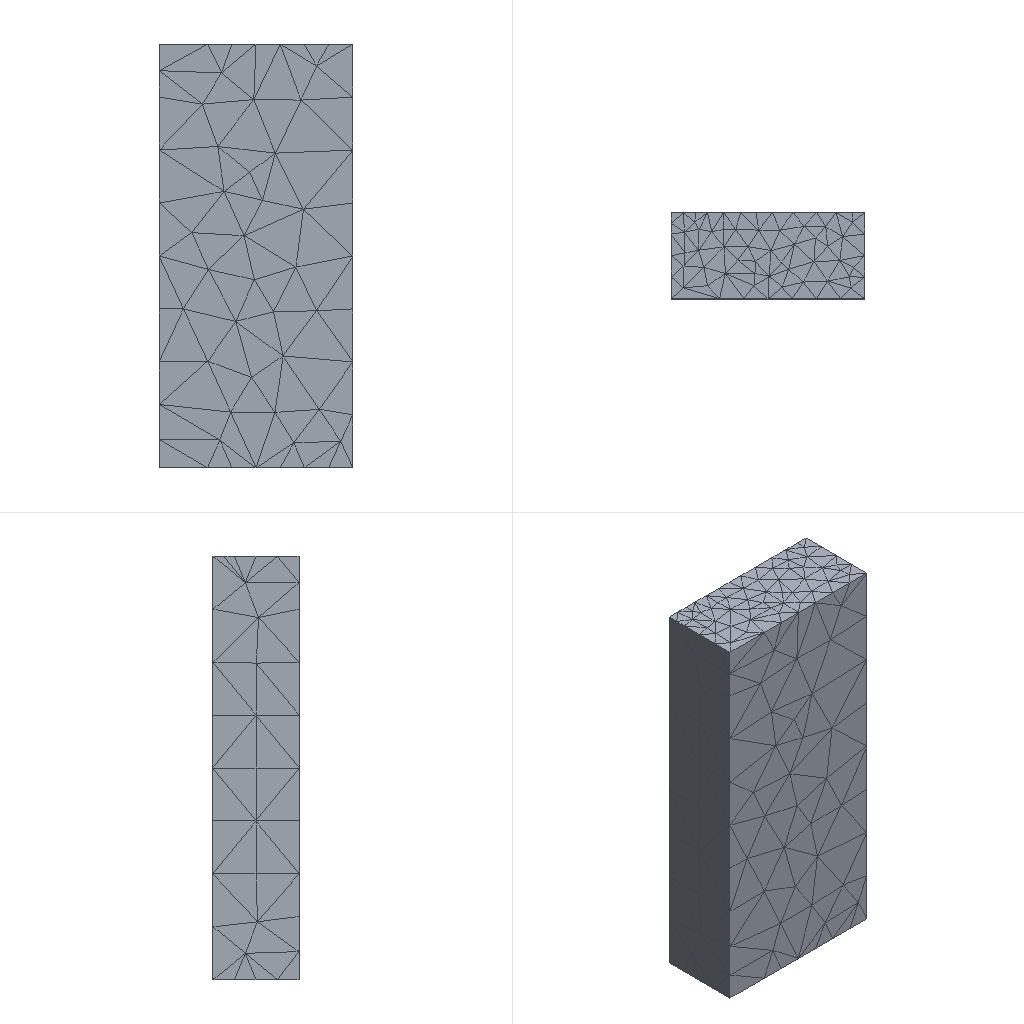Simulation study | ansys electronics desktop
Set-up summary:
category,name,step,type,value,unit,region
solver,ansys_electronics_desktop
units,length mm,,stated,model units
analysis,DESIGN_1,,HFSS Modal Network,design_type=HFSS
setup,Setup1,DESIGN_1,HfssDriven,frequency=10GHz; max_passes=6; max_delta_s=0.02
sweep,Sweep1,Setup1,Discrete,8GHz..12GHz n=9 step=
mesh,nodes,,,n/a (no mesh stored)
mesh,elements,,,n/a (no mesh stored)
material,vacuum,,permittivity,1
load,1,DESIGN_1,wave port,,,faces 8
load,2,DESIGN_1,wave port,,,faces 7
bc,PerfE,DESIGN_1,perfect e,,,"faces 9, 10, 11, 12"
Ansys Electronics Desktop project file, long lists of numbers shortened, first 452 of 1466 lines:
$begin 'AnsoftProject'
	Created='Fri Sep  4 17:09:57 2026'
	Product='ElectronicsDesktop'
	FileOwnedByWorkbench=false
	$begin 'Desktop'
		Version(2026, 1)
		InfrastructureVersion(1, 0)
		$begin 'FactoryHeader'
			$begin 'geometry3deditor'
				KernelVersion(2, 0)
				ProjectContainsGeometry3D='1'
			$end 'geometry3deditor'
		$end 'FactoryHeader'
	$end 'Desktop'
	UsesAdvancedFeatures=false
	PreviewImageDesignId=1
	NextUniqueID=0
	MoveBackwards=false
	$begin 'HFSSEnvironment'
		Version(1, 0)
	$end 'HFSSEnvironment'
	$begin 'PlanarEMEnvironment'
		Version(1, 0)
	$end 'PlanarEMEnvironment'
	$begin 'Q3DEnvironment'
		Version(1, 0)
	$end 'Q3DEnvironment'
	$begin '2DExtractorEnvironment'
		Version(1, 0)
	$end '2DExtractorEnvironment'
	$begin 'NexximEnvironment'
		Version(1, 0)
	$end 'NexximEnvironment'
	$begin 'NexximNetlistEnvironment'
		Version(1, 0)
	$end 'NexximNetlistEnvironment'
	$begin 'EmitEnvironment'
		Version(1, 0)
	$end 'EmitEnvironment'
	$begin 'Maxwell3DEnvironment'
		Version(1, 0)
	$end 'Maxwell3DEnvironment'
	$begin 'Maxwell2DEnvironment'
		Version(1, 0)
	$end 'Maxwell2DEnvironment'
	$begin 'RMxprtEnvironment'
		Version(1, 0)
	$end 'RMxprtEnvironment'
	$begin 'MaxCirEnvironment'
		Version(1, 0)
	$end 'MaxCirEnvironment'
	$begin 'SimplorerEnvironment'
		Version(1, 0)
	$end 'SimplorerEnvironment'
	$begin 'IcepakEnvironment'
		Version(1, 0)
	$end 'IcepakEnvironment'
	$begin 'IcepakFEAEnvironment'
		Version(1, 0)
	$end 'IcepakFEAEnvironment'
	$begin 'SchematicEnvironment'
		Version(1, 0)
	$end 'SchematicEnvironment'
	$begin 'geometry3deditor'
		Version(1, 0)
	$end 'geometry3deditor'
	ReadVersion=12
	$begin 'DesignMgrEnvironment'
		CompInstCounter=1
		GPortCounter=0
		NetCounter=0
		Alias('Ieee;Simplorer Elements\\Ieee', 'Std;Simplorer Elements\\Std', 'Basic_VHDLAMS;Simplorer Elements\\Basic Elements VHDLAMS\\Basic Elements VHDLAMS', 'Digital_Elements;Simplorer Elements\\Digital Elements\\Digital Elements', 'Transformations;Simplorer Elements\\Tools\\Transformations\\Transformations', 'HEV_VHDLAMS;Simplorer Elements\\HEV VHDLAMS\\HEV VHDLAMS', 'automotive_vda;Simplorer Elem
	$end 'DesignMgrEnvironment'
	$begin 'ProjectDatasets'
		NextUniqueID=0
		MoveBackwards=false
		DatasetType='ProjectDatasetType'
		$begin 'DatasetDefinitions'
		$end 'DatasetDefinitions'
	$end 'ProjectDatasets'
	VariableOrders[0:]
	$begin 'Definitions'
		$begin 'Materials'
			$begin 'vacuum'
				CoordinateSystemType='Cartesian'
				BulkOrSurfaceType=1
				$begin 'PhysicsTypes'
					set('Electromagnetic')
				$end 'PhysicsTypes'
				$begin 'AttachedData'
					$begin 'MatAppearanceData'
						property_data='appearance_data'
						Red=230
						Green=230
						Blue=230
						Transparency=0.95
					$end 'MatAppearanceData'
				$end 'AttachedData'
				permittivity='1'
				ModTime=1499970477
				Library='Materials'
				LibLocation='SysLibrary'
				ModSinceLib=false
			$end 'vacuum'
		$end 'Materials'
		$begin 'SurfaceMaterials'
			$begin 'Steel-oxidised-surface'
				CoordinateSystemType='Cartesian'
				BulkOrSurfaceType=2
				$begin 'PhysicsTypes'
					set('Thermal')
				$end 'PhysicsTypes'
				surface_emissivity='0.8'
				ModTime=1461288057
				Library='SurfaceMaterials'
				LibLocation='SysLibrary'
				ModSinceLib=false
			$end 'Steel-oxidised-surface'
		$end 'SurfaceMaterials'
		$begin 'Scripts'
		$end 'Scripts'
		$begin 'AnsysComponents'
			NextUniqueID=0
			MoveBackwards=false
			$begin 'AnsysComponentDefinitions'
			$end 'AnsysComponentDefinitions'
		$end 'AnsysComponents'
		$begin 'Symbols'
			$begin 'DESIGN_1'
				ModTime=1788512998
				Library=''
				ModSinceLib=false
				LibLocation='Project'
				HighestLevel=1
				Normalize=true
				InitialLevels(0, 1)
				$begin 'Graphics'
					Rect(0, 0, 0, 0, 0.00254, 0.00254, 0.00508, 0.00508, 0, 0, 0)
					Rect(0, 1, 0, 0, 0.0004233, 0.00254, 0.0004233, 0.0004233, 0, 0, 0)
				$end 'Graphics'
			$end 'DESIGN_1'
		$end 'Symbols'
		$begin 'DefInfo'
			DESIGN_1(1002, 0, 0, 0, '', 1788512998, '', 'DESIGN_1', '', '', '', '', '', 'Design.bmp', '', 'Project', '', '', 1788512998, '', 0, 0)
		$end 'DefInfo'
		$begin 'Compdefs'
			$begin 'DESIGN_1'
				Library=''
				CircuitEnv=0
				Refbase='U'
				NumParts=1
				ModSinceLib=true
				$begin 'Properties'
					TextProp('Representation', 'SRD', '', 'DESIGN_1')
					TextProp('Owner', 'SRD', '', 'HFSS')
				$end 'Properties'
				CompExtID=6
				$begin 'Parameters'
					ButtonProp('CosimDefinition', 'D', '', 'Edit', 'Edit', 40501, ButtonPropClientData())
					MenuProp('CoSimulator', 'D', '', 'DefaultNetlist', 0)
				$end 'Parameters'
				$begin 'CosimDefinitions'
					$begin 'CosimDefinition'
						CosimulatorType=4
						CosimDefName='DefaultNetlist'
						IsDefinition=true
						Connect=true
						Data()
						GRef()
					$end 'CosimDefinition'
					DefaultCosim='DefaultNetlist'
				$end 'CosimDefinitions'
			$end 'DESIGN_1'
		$end 'Compdefs'
	$end 'Definitions'
	DesignIDServer=2
	MoveBackwards=false
	$begin 'HFSSModel'
		RepRewriteV2=true
		Name='DESIGN_1'
		DesignID=0
		'Use Advanced DC Extrapolation'=false
		'Use Power S'=false
		'Export FRTM After Simulation'=false
		'Export Rays After Simulation'=false
		'Export After Simulation'=false
		'Allow Material Override'=false
		'Calculate Lossy Dielectrics'=false
		'Perform Minimal validation'=false
		$begin 'TemperatureSettings'
			IncludeTemperatureDependence=false
			EnableFeedback=false
			Temperatures(6, '22cel')
		$end 'TemperatureSettings'
		ObjsEnabledForDeformation()
		'Port Validation Settings'='Standard'
		'Save Adaptive support files'=false
		SolutionType='HFSS Modal Network'
		$begin 'DrivenOptions'
			AutoOpen=false
		$end 'DrivenOptions'
		HasTransientSetups=false
		MaterialDensity=1
		MassOfTissue=1
		VoxelSize=1
		TissueObjectList=-1
		AverageSarMethod=0
		UseAutoDCThickness=true
		HaveZwaveSupport=true
		SolveInsideThreshold=100000
		RequireBodyFaceInfo=false
		$begin 'OutputVariable'
			NextUniqueID=0
			MoveBackwards=false
		$end 'OutputVariable'
		$begin 'ModelSetup'
			$begin 'DesignDatasets'
				NextUniqueID=0
				MoveBackwards=false
				DatasetType='DesignDatasetType'
				$begin 'DatasetDefinitions'
				$end 'DatasetDefinitions'
			$end 'DesignDatasets'
			VariableOrders[0:]
			$begin 'Editor3D Doc Preferences'
				BackgroundColorVersion=1
				'Plane Background'=0
				'Need Lights'=true
				'Ambient Light'=8355711
				'Num Lights'=1
				Light0[4: 16777215, 0.75, -0.15, -0.63]
				Ver=2
			$end 'Editor3D Doc Preferences'
			SnapMode=31
			WorkingCS=1
			$begin 'GeometryCore'
				BlockVersionID=3
				DataVersion=3
				NativeKernel='PARASOLID'
				NativeKernelVersionID=26
				Units='mm'
				ModelExtents=10000
				InstanceID=-1
				$begin 'ValidationOptions'
					EntityCheckLevel='Strict'
					IgnoreUnclassifiedObjects=false
					SkipIntersectionChecks=false
				$end 'ValidationOptions'
				ContainsGeomLinkUDM=false
				$begin 'GeometryOperations'
					BlockVersionID=2
					$begin 'AnsoftRangedIDServerManager'
						$begin 'AnsoftRangedIDServer'
							IDServerObjectTypeID=0
							IDServerRangeMin=0
							IDServerRangeMax=2146483647
							NextUniqueID=36
							MoveBackwards=false
						$end 'AnsoftRangedIDServer'
						$begin 'AnsoftRangedIDServer'
							IDServerObjectTypeID=1
							IDServerRangeMin=2146483648
							IDServerRangeMax=2146485547
							NextUniqueID=2146483654
							MoveBackwards=false
						$end 'AnsoftRangedIDServer'
					$end 'AnsoftRangedIDServerManager'
					StartBackGroundFaceID=2146483648
					$begin 'CoordinateSystems'
					$end 'CoordinateSystems'
					$begin 'OperandCSs'
					$end 'OperandCSs'
					$begin 'SubModelDefinitions'
					$end 'SubModelDefinitions'
					$begin 'Groups'
					$end 'Groups'
					$begin 'UserDefinedModels'
					$end 'UserDefinedModels'
					$begin 'OperandUserDefinedModels'
					$end 'OperandUserDefinedModels'
					$begin 'ToplevelParts'
						$begin 'GeometryPart'
							$begin 'Attributes'
								Name='WG'
								Flags=''
								Color='(230 230 230)'
								Transparency=0.8
								PartCoordinateSystem=1
								UDMId=-1
								GroupId=-1
								MaterialValue='"vacuum"'
								SurfaceMaterialValue='""'
								SolveInside=true
								ShellElement=false
								ShellElementThickness='0mm'
								ReferenceTemperature='20cel'
								IsMaterialEditable=true
								IsSurfaceMaterialEditable=true
								UseMaterialAppearance=false
								IsLightweight=false
								IsAlwaysHidden=false
							$end 'Attributes'
							$begin 'PhysicsAttributes'
								SuppressedForPhysics='False'
								SuppressedForPhysicsEditable=true
							$end 'PhysicsAttributes'
							$begin 'Operations'
								$begin 'Operation'
									OperationType='Box'
									ID=5
									ReferenceCoordSystemID=1
									$begin 'BoxParameters'
										KernelVersion=24
										XPosition='0mm'
										YPosition='0mm'
										ZPosition='0mm'
										XSize='22.86mm'
										YSize='10.16mm'
										ZSize='50mm'
									$end 'BoxParameters'
									ParentPartID=6
									ReferenceUDMID=-1
									IsSuppressed=false
									$begin 'OperationIdentity'
										$begin 'Topology'
											NumLumps=1
											NumShells=1
											NumFaces=6
											NumWires=0
											NumLoops=6
											NumCoedges=24
											NumEdges=12
											NumVertices=8
										$end 'Topology'
										BodyID=6
										StartFaceID=7
										StartEdgeID=13
										StartVertexID=25
										NumNewFaces=6
										NumNewEdges=12
										NumNewVertices=8
										FaceNameAndIDMap()
										EdgeNameAndIDMap()
										VertexNameAndIDMap()
									$end 'OperationIdentity'
								$end 'Operation'
							$end 'Operations'
							$begin 'SubregionDependencyInformation'
								ChildSubregions[0:]
							$end 'SubregionDependencyInformation'
						$end 'GeometryPart'
					$end 'ToplevelParts'
					$begin 'OperandParts'
					$end 'OperandParts'
					$begin 'Planes'
					$end 'Planes'
					$begin 'Points'
					$end 'Points'
					$begin 'GeometryEntityLists'
					$end 'GeometryEntityLists'
					$begin 'CachedNames'
						$begin 'allobjects'
							allobjects(-1)
						$end 'allobjects'
						$begin 'global'
							global(-1)
						$end 'global'
						$begin 'model'
							model(-1)
						$end 'model'
						$begin 'wg'
							wg(-1)
						$end 'wg'
					$end 'CachedNames'
				$end 'GeometryOperations'
				$begin 'GeometryDependencies'
					$begin 'DependencyInformation'
						NumParents=1
						DependencyObject('GeometryBodyOperation', 5)
						DependencyObject('CoordinateSystem', 1)
					$end 'DependencyInformation'
				$end 'GeometryDependencies'
			$end 'GeometryCore'
			$begin 'AssignedEntities'
				AssignedObject[1: 6]
				$begin 'AssignedFace'
					kID=7
					$begin 'FaceData'
						ParentObjectID=6
						NormalValid=false
						$begin 'FaceGeomTopol'
							FaceTopol(1, 4, 4, 4)
							$begin 'FaceGeometry'
								Area=232.258
								FcUVMid(11.43, 5.08, 50)
								$begin 'FcTolVts'
									TolVt(22.86, 0, 50, 5e-07)
									TolVt(22.86, 10.16, 50, 5e-07)
									TolVt(0, 10.16, 50, 5e-07)
									TolVt(0, 0, 50, 5e-07)
								$end 'FcTolVts'
							$end 'FaceGeometry'
						$end 'FaceGeomTopol'
					$end 'FaceData'
				$end 'AssignedFace'
				$begin 'AssignedFace'
					kID=8
					$begin 'FaceData'
						ParentObjectID=6
						NormalValid=false
						$begin 'FaceGeomTopol'
							FaceTopol(1, 4, 4, 4)
							$begin 'FaceGeometry'
								Area=232.258
								FcUVMid(11.43, 5.08, 0)
								$begin 'FcTolVts'
									TolVt(22.86, 0, 0, 5e-07)
									TolVt(0, 0, 0, 5e-07)
									TolVt(0, 10.16, 0, 5e-07)
									TolVt(22.86, 10.16, 0, 5e-07)
								$end 'FcTolVts'
							$end 'FaceGeometry'
						$end 'FaceGeomTopol'
					$end 'FaceData'
				$end 'AssignedFace'
				$begin 'AssignedFace'
					kID=9
					$begin 'FaceData'
						ParentObjectID=6
						NormalValid=false
						$begin 'FaceGeomTopol'
							FaceTopol(1, 4, 4, 4)
							$begin 'FaceGeometry'
								Area=1143
								FcUVMid(11.43, 0, 25)
								$begin 'FcTolVts'
									TolVt(22.86, 0, 50, 5e-07)
									TolVt(0, 0, 50, 5e-07)
									TolVt(0, 0, 0, 5e-07)
									TolVt(22.86, 0, 0, 5e-07)
								$end 'FcTolVts'
							$end 'FaceGeometry'
						$end 'FaceGeomTopol'
					$end 'FaceData'
				$end 'AssignedFace'
				$begin 'AssignedFace'
					kID=10
					$begin 'FaceData'
						ParentObjectID=6
						NormalValid=false
						$begin 'FaceGeomTopol'
							FaceTopol(1, 4, 4, 4)
Last 416 lines:
				$end 'RegularArray'
				$begin 'CustomArray'
					NumCells=0
					$begin 'Cell'
					$end 'Cell'
				$end 'CustomArray'
				$begin 'ParametricArray'
					DesignFrequency='1GHz'
					LayoutType=1
					CenterCellX='0mm'
					CenterCellY='0mm'
					CenterCellZ='0mm'
					SpecifyDesignInWavelength=true
					WidthSpacing='14.99mm'
					WidthSpacingInWavelength='0.05'
					Width='119.917mm'
					WidthInWavelength='0.4'
					LengthSpacing='14.99mm'
					LengthSpacingInWavelength='0.05'
					Length='89.938mm'
					LengthInWavelength='0.3'
					SymmetryType=0
					StaggerAngle='0deg'
					StaggerType=0
					UDirnX='1'
					UDirnY='0'
					UDirnZ='0'
					VDirnX='0'
					VDirnY='1'
					VDirnZ='0'
					WeightType=3
					EdgeTaperX_db='-200'
					CosineExp='1'
					DifferentialType=0
					Behavior='UseScanAngle'
					ScanAnglePhi='45deg'
					ScanAngleTheta='45deg'
					UDirnPhaseShift='0deg'
					VDirnPhaseShift='0deg'
				$end 'ParametricArray'
			$end 'ArraySetup'
			$begin 'NearFieldSetups'
				NextUniqueID=0
				MoveBackwards=false
			$end 'NearFieldSetups'
			RadFieldComputationVersion=1.8
			RadfieldHeaderFile='RAD6E3F2452017885130237.tmp'
			RadPowerMethod=0
		$end 'RadField'
		$begin 'SolutionManager'
			$begin 'SimSetup'
				TypeName='BaseSetup'
				ID=6
				Name='Setup1'
				$begin 'Solution'
					ID=7
					Name='AdaptivePass'
					$begin 'SimDataExtractor'
						IsPortOnly=false
					$end 'SimDataExtractor'
				$end 'Solution'
				$begin 'Solution'
					ID=8
					Name='LastAdaptive'
					$begin 'SimDataExtractor'
						$begin 'Sweeps'
							$begin 'Sweep'
								Variable='Freq'
								Column='10GHz'
								Units='GHz'
							$end 'Sweep'
							$begin 'PostprocessSweep'
								Variable='NormalizedDistance'
								RegularSweep=1
								Units=''
								Minimum=0
								Maximum=1
								Increment=0.01
								CreateIndexedSubsweepFlag=false
							$end 'PostprocessSweep'
							$begin 'PostprocessSweep'
								Variable='Phi'
								RegularSweep=1
								Units='deg'
								Minimum=0
								Maximum=6.283
								Increment=0.08727
								CreateIndexedSubsweepFlag=false
							$end 'PostprocessSweep'
							$begin 'PostprocessSweep'
								Variable='Theta'
								RegularSweep=1
								Units='deg'
								Minimum=0
								Maximum=6.283
								Increment=0.08727
								CreateIndexedSubsweepFlag=false
							$end 'PostprocessSweep'
							$begin 'PostprocessSweep'
								Variable='Phase'
								RegularSweep=1
								Units='deg'
								Minimum=0
								Maximum=6.283
								Increment=0.08727
								CreateIndexedSubsweepFlag=false
							$end 'PostprocessSweep'
						$end 'Sweeps'
						IsPortOnly=false
					$end 'SimDataExtractor'
				$end 'Solution'
				$begin 'Solution'
					ID=14
					Name='Sweep1'
					$begin 'SimDataExtractor'
						IsPortOnly=false
					$end 'SimDataExtractor'
				$end 'Solution'
			$end 'SimSetup'
			$begin 'Version ID Map'
				V=1
				$begin 'Setup'
					N='Setup1'
					V=0
					Soln(N='AdaptivePass', V=0)
					Soln(N='LastAdaptive', V=12)
					Soln(N='Sweep1', V=0)
				$end 'Setup'
				IQM=0
			$end 'Version ID Map'
			$begin 'ID Map'
				$begin 'Setup'
					N='Setup1'
					I=6
					Soln(N='AdaptivePass', I=7)
					Soln(N='LastAdaptive', I=8)
					Soln(N='Sweep1', I=14)
				$end 'Setup'
			$end 'ID Map'
			ValidationCacheHeader=''
		$end 'SolutionManager'
		$begin 'UserDefinedSolutionMgr'
			NextUniqueID=1000000
			MoveBackwards=false
		$end 'UserDefinedSolutionMgr'
		$begin 'DatasetSolutionMgr'
			NextUniqueID=2000000
			MoveBackwards=false
		$end 'DatasetSolutionMgr'
		Notes=$begin_cdata$ $end_cdata$
		$begin 'AnimationSetups'
		$end 'AnimationSetups'
		CacheHeaderFile='HDR6E3F2452017885130238.tmp'
	$end 'HFSSModel'
	$begin 'DataInstances'
		DesignEditor='TopLevel'
		Refdes('0', 'U1')
		$begin 'CompInstances'
			$begin 'Compinst'
				ID='0'
				Status='Status'
				CompName='DESIGN_1'
				GatesInUse()
				$begin 'Properties'
					TextProp('ID', 'SRID', '', '0')
				$end 'Properties'
				$begin 'Parameters'
					MenuProp('CoSimulator', 'OHD', '', 'DefaultNetlist', 0)
					ButtonProp('CosimDefinition', 'OHD', '', 'Edit', 'Edit', 40501, ButtonPropClientData())
				$end 'Parameters'
			$end 'Compinst'
		$end 'CompInstances'
		$begin 'Instance'
			DesignEditor='DESIGN_1'
			ID='0'
			$begin 'HfssDesignInstance'
				DesignInstanceID=1
				$begin 'WindowPosition'
					$begin 'EditorWindow'
						Circuit(Editor3d(View('View Orientation Gadget'=1, WindowPos(3, -1, -1, -8, -31, 26, 26, 1631, 489), OrientationMatrix(0.02344, -0.01353, 0.01914, 0, 0.02344, 0.01353, -0.01914, 0, 0, 0.02706, 0.01914, 0, -0.387, -0.5907, -6.194, 1, 0, -2.542, 2.542, -1, 
					$end 'EditorWindow'
				$end 'WindowPosition'
				$begin 'ReportSetup'
					$begin 'ReportManager'
						$begin 'Reports'
						$end 'Reports'
						NextUniqueID=0
						MoveBackwards=false
						$begin 'NextVersID'
							NextUniqueID=0
							MoveBackwards=false
						$end 'NextVersID'
					$end 'ReportManager'
					$begin 'Reports'
					$end 'Reports'
					$begin 'ReportsWindowInfoList'
					$end 'ReportsWindowInfoList'
				$end 'ReportSetup'
				$begin 'Properties'
				$end 'Properties'
				$begin 'UserDefinedDocument'
					$begin 'Data'
					$end 'Data'
				$end 'UserDefinedDocument'
			$end 'HfssDesignInstance'
		$end 'Instance'
		$begin 'SODInfo'
			$begin 'DESIGN_1'
				$begin 'CosimDefinition'
					CosimDefName='DefaultNetlist'
					$begin 'SODInstanceMap'
					$end 'SODInstanceMap'
					SODComponentList()
				$end 'CosimDefinition'
			$end 'DESIGN_1'
		$end 'SODInfo'
	$end 'DataInstances'
	$begin 'WBSystemIDToDesignInstanceIDMap'
	$end 'WBSystemIDToDesignInstanceIDMap'
	$begin 'WBSysIDSysDetails'
	$end 'WBSysIDSysDetails'
	$begin 'WBConnIDConnDetails'
	$end 'WBConnIDConnDetails'
	$begin 'WBMaterialGuidDetails'
		WBMaterialGuidMap()
	$end 'WBMaterialGuidDetails'
	$begin 'MinervaProjectSettingsBlk'
		MinervaRemoteFilePath=''
		FolderContainerString=''
	$end 'MinervaProjectSettingsBlk'
$end 'AnsoftProject'
$begin 'AllReferencedFilesForProject'
$end 'AllReferencedFilesForProject'
$begin 'ProjectPreview'
	ProductName='ElectronicsDesktop'
	MajorVersion=2026
	MinorVersion=1
	IsEncrypted=false
	Thumbnail64='/9j/4AAQSkZJRgABAQAAAQABAAD/2wBDAAEBAQEBAQEBAQEBAQEBAQEBAQEBAQEBAQEBAQEBAQEBAQE\
BAQICAQECAQEBAgICAgICAgICAQICAgICAgICAgL/2wBDAQEBAQEBAQEBAQECAQEBAgICAgICAgICAg\
ICAgICAgICAgICAgICAgICAgICAgICAgICAgICAgICAgICAgICAgL/wAARCABgAGADASIAAhEBAxEB/\
8QAHwAAAQUBAQEBAQEAAAAAAAAAAAECAwQFBgcICQoL/8QAtRAAAgEDAwIEAwUFBAQAAAF9AQIDAAQR\
BRIhMUEGE1FhByJxFDKBkaEII0KxwRVS0fAkM2JyggkKFhcYGRolJicoKSo0NTY3ODk6Q0RFRkdISUp\
TVFVWV1hZWmNkZWZnaGlqc3R1dnd4eXqDhIWGh4iJipKTlJWWl5iZmqKjpKWmp6ipqrKztLW2t7i5us\
LDxMXGx8jJytLT1NXW19jZ2uHi4+Tl5ufo6erx8vP09fb3+Pn6/8QAHwEAAwEBAQEBAQEBAQAAAAAAA\
AECAwQFBgcICQoL/8QAtREAAgECBAQDBAcFBAQAAQJ3AAECAxEEBSExBhJBUQdhcRMiMoEIFEKRobHB\
CSMzUvAVYnLRChYkNOEl8RcYGRomJygpKjU2Nzg5OkNERUZHSElKU1RVVldYWVpjZGVmZ2hpanN0dXZ\
3eHl6goOEhYaHiImKkpOUlZaXmJmaoqOkpaanqKmqsrO0tba3uLm6wsPExcbHyMnK0tPU1dbX2Nna4u\
Pk5ebn6Onq8vP09fb3+Pn6/9oADAMBAAIRAxEAPwD+rnTfH/7fXxx/aA/bO8I/BT43fsgfB/4Zfsz/A\
LQHgn4F+GdH+KX7HPxo+OvjvxF/bf7IH7LP7SGs+Kdd8b+E/wBvL4e6fHu8QftB6rp1rY2/hyP7PZ+H\
Ld5by6nmkZfQP+Fc/wDBU3/o8j9gD/xWn+0V/wDTYq/Er/goPrX7Z3hTV/2tvHv7EOj/ALQnif4g/C7\
/AILq/Ar4wfEHwV+zvbfETUNY+I3wl+D/APwQr/Zp+J+q/C34h6P8Oo3l8RfDLxT448J+APDtxpWpRz\
aZqur+JtG05oZr+6sIn8I+Cn7Qv/BZf9k74Jfs6eDPFp/aP8YRfDf9nj/gpV4n+OPxJ/ap+HWu6n4Iu\
/G3w21f/gqj4z+BHjX42/tL/Fbw1d3nh3RftvwR/ZEi02bV/FvgvQ7Hwn8RdINpB41sPFtnc+AwD+iz\
/hXP/BU3/o8j9gD/AMVp/tFf/TYqP+Fc/wDBU3/o8j9gD/xWn+0V/wDTYq8t/wCCVXx5+K3x18K/tbD\
4n/FL4s/F2y+FP7Vmi/DX4ZeKvjn8EvCX7PnxWT4f3v7GX7H/AMWbjT/GPwz8I/D7wwmk6gfiP8U/iH\
dq15pMN6YdViiZYbWG1tLb5v8A+Ca+k/GWy/bC/a98RfG34n/tOX2oz/Fz9vKPQ/hr8afgj/wVO8PfD\
nwx8L4f24/E5+COu+Bfj18ev2htR/Zp8Y+HG+CNn4Hk8Mad8Nvh1oHiCHwxrkMdtq81npPi6XWgD7i/\
4Vz/AMFTf+jyP2AP/Faf7RX/ANNio/4Vz/wVN/6PI/YA/wDFaf7RX/02Kv8APS+EuqftaXnhTwt+33q\
kX7SnxA+InwL8SfA+81r9oLxdffEz4weD4/FXww0jwPpPjeX4n/HXx/rmp3eneL7vxz4t+EzaR4eubx\
re60vxZrVtplva6RoKWcf7pfCj/gpF/wAFK/2M/gZ8F/2kvj14++NP7Q37PFpqPg3wl4b8D/GT4ceC/\
h1/wuzwh49+I/8AwVN+Gvgm40/9o+4+Ds/iLxH4h0n4Tfsm/sY/EFdYu7rXtV1/TvjlPqWv3Wo23i/Q\
NXtAD93P2sfFv/BU39l/9lj9pb9pf/hqD9gDxx/wzv8As/8Axk+On/CFf8O7v2ivDP8AwmH/AAqT4de\
I/H//AAi3/CR/8PS9Q/4R/wDtD/hH/sn277BffZPtfn/Y7ny/Jf8AX6v4pfjT/wAFLfi34D/4JRftIf\
Bbxf8AsxftDeNPgD+03pv/AAVT/Zp/Zz/au+L37Qmp/Ev4kSXPjT4tftXeDPhV8L/iloXxRvta8XWet\
eCdGudJ8H3z+J/FE+py2/wtvrjTm1O3tY9/7y/tDf8ABUfxJ4J/a51b9h39lr9lPxN+1n+0N4P8G2Xj\
n4gaEfiz4J+BXhvwzpGo6RoPiG2trHxT48065i8R6ougeKPDl3PHDHHEia1FFFNPPFexWgB+utFfij8\
VP+CtfxU+Ev7Hnjb9p/xj/wAE+/jp4F8U/Cb4r+Fvh58VvhL8XNU1j4Z2GneHPFc2paRZfEr4cfFO5+\
GN9YfFbwyviyPQtLb7FZWyiXXUuHnjtmsZNR9x/bR/4KWaD+zH8Pv2UPE/wt+GX/DQ/i/9svx14N8Lf\
BXwLB46X4eHXdD8ZaNpupWnixddTwhrxkgjvfE/ga1Nulkd58VpKbhBDslAP09or8V/F/8AwVo+JHir\
9oj4+fs9/sY/sQeMP2uNS/Zg1KbQ/jT4iT43fD/4NRaRrdjf6ppGrWHhLQfFWkX1541+za3omsWGLdY\
ria70yRIbZ4ZLWe4/SD9lr496j+0l8HtD+J2t/Bf4xfs/eILy7vtK8QfCz44+CNe8DeNfD2r6a0QuDF\
aa9ptq2u+Hpo54JbLU7eIQXMchR0gu4Lq1twD8Z/Efx6+K/wCzv+1f+3fqWmftd/st/s2+Avj1/wAFV\
v2cP2Xvh1ovxx/Yi/aD/ad8R+Nf2lvib/wS8/YFvvCmjWvjf4Nftf8AgSy8EeGtR0HQBGja1oaadps+\
gXd3qPidYtQtLOz3PBP7ePij43fB34ffEu2/4LA/8EeLf4V/tAeH/iHP8P7X41fsB/HD4M6h8SvCngX\
xT4v+G3xHuLT4afHb/grBoOtaj4cs/EfgvxjYXslxpItZItInlBls2SZ/jT9ur4V/DX9qT4o/t8/ADx\
L8Qf2pPhB4z+GP/BVP4U/tQ+EPiL8Dv+CcH7Z/7bvhy112z/4Iq/sr/BfwXBda/wDs6/Dm80PQPEul+\
L/iHa+I30+61xNVEHhC0im061tdesdWi8Mvv2QPBFj8BvgF+zh4F/a5/wCCiHhr4S/s+ePG+KnhjwBq\
v/BCP/grfrXw81X4i2P7ePj79tDRNc8TfDzRPBujaV4303+xPGWjeDNQ07xPb+IbZh4C03xHoP8Awjd\
3NqWn3wB92fET9mT4Vf8ACl1bxj8T/wDg33+IXwY/Z9ifxJongrw5/wAEU9Y+NWm/Di4+OHxQ1L4QrP\
8AD74UeBP+ClOtXlr4h8a/Gv4Uav4WgttC0l9Q8U+K/hrc6FBDqGsaNLaW3hf7Z3/BUn43WH7Jvxr1L\
wZ+3Z+yr8XH1jRtQ+D2o6H8O/8Aglb+278DNZ0vxl4xk/4RPxh8Mpvjl8UP23db8NfBv9o/w94Y1LWd\
bvPBuv6Xd+MdKt9D+1X3hWK3P2hPqj4RfGFP2d/2HtC/Y2+BHxj/AGxfBOofDD4MeB/hD8CvjZqv/BA\
L/gqV4j8TeCW8K+MvFX9peLfG/hCD4SWGkfEfVrv4QXHgHRoVgj0F4PE3h7W/GF9catD4gtfDOgfnx4\
9/Y8/Zr+Mf/CFzfFTXP2kLe4+H/jbwh8cdM0z4S/8ABBz/AILueE/AvxA/aR+Hsd1o3hj4pfHj4a/FX\
x9480T4rwaj4Mey0zxrOLPSvHvjRbBX1T4jR2whsYADz/8AZs/4JJePfiT8HvhX+zlaf8FTvi58GfGX\
7Rn7OviP9qDU/wBhXVfg38avDGiWfg/Q/EngHwb431Hx54P1v4vaLarpsPxC8Y+C9MTUdU8PWza+0T6\
joNtq+nadPdQ/nD8cP2gvjF4p/wCCXXw//Zh+K3xZ+Eduf2Y/2wp/hzpP7Pk3wu8Taf8AtE2MHh3wN8\
U7yXx9rHxeuPjpdaT4g+Hmk6n401rwy2jW/wAPdPurSZdIaTxE6Qm31D+lj4MeK/gv8BR8DNc+Hus/t\
mWnjP4Cfs3/ALdXwX8HW13/AMEMf+Cry/CTTfFf7Zvx6+Av7QOhaj4d+GWj/Bmzu/CfwG+H2ufBCDw/\
4e+Htp4iNwfCOo6fo1v4w0uTRlvr784vj5+xz8Etc1/9rD4p/Bv4jft3+N/iD+0D8cP2jfjP4B8BftQ\
/8EXf+Cl+s+AfgPqv7WOg/s9WfxX8S/CL4jfDr9iK08UeCPjxoviv9nzwXqfw/wDG11H4hsvB+neDtA\
0ay8HvrUWu+NdfAPFP+CnXj628Q/8ABPX4c/Dz4WfGb9jjxB+z98Mv2h/hbrvhT4N/sw/8Eyv2hv8Ag\
n3Y6LZ/GfwF+074o8D/ABg8AyfF79pjxNovj74G+Kbrw78W7ix1fwt4afRvE+qi61Sx8UytYX9vf+4/\
8FjLT9j1v+ChXxFvPjZN8f8A4FfEjSfCPw/8ReHfjv8ACHS7TUdO8RTaZ8P/AA1/Y9lLZwapPcXHiWN\
0nsbWcR6AYW0uFbvUvsYgnHxz4v8A2y/hp+yd+wT/AMFSvhf4J8La38R9N+L/AMJfAH7GL/Fbw1+zD8\
dv2Z/AXxN1iT4C/HW1/aF+Ofxotfib4OebTP2+biTxtq1j4rn8XXum6/42bwd4f1m08P3Gk+HNZkr6I\
/aG/aN+NPxO+Nf7QXj3XF+Cvgfxv8I/jt49+FHxg8UjT/Fg8FSaj8ANM0fwHD4s8KeFbjWZLryNQi8O\
adM9vqGuSNZRny0mv8JGPpeF8HSx+MxeFqyhGNTDz1lS9rqqlJ3jHnpcskk3z+0goxUnKXLdP8D+kJ4\
gY7wz4c4Q4qweCrZhTo8QYShiKVLGrAxlQxGCzGm1Wm8NjHXg6rpRp4SGFr1cTipYenRUKrhWp/on/w\
AEkrr9pH/goH+wp+2x8AP2qfGniD4n/CTUpLj4OfA74veP7e9uPGd/Nq/hPVdSv9Svb7WreLVNdtdHm\
vfhbrul3eqRy3gm1uSBp5I7ZLe2+Lf+CPXh/wCMP7WP7Z/wF8J/HXRZ7fw3/wAEjvg544+Ho0++eS7i\
PxX1H4j+M/DvhC21GF0A0/VbDRmgt7dUJUf8KNtZiS0jRr6Pp/8AwUr+MfgL/gk58Zvjn8JLK6+G37R\
fxF+NfhrXrS40nTtD1yH4a+AfC3hP9kT4eeLPiVNpPjfSb+0vvDOqXuv+DtFso7iCact8V7W6tmY2M1\
xF9weK/h/qf/BE34D/AAz1D4dfFjwF45+Kf7Zn7fnwu8B/tL/tP/tO+FtRm8N6Zo/xP0f4iahrvxHvv\
Dvh34q+Hv7M03QJtGudVkGoeJnhb+1talu76JbqGWw+cnFRnOKlzKLaTs1dJ72eqv2eqP3qEnKEZOPK\
5JNq6dm1tdaO3daHwj/wUW+HH/BOTQP2wPjL438UeMv25f8AgnH+1FZaheeKdH+L3hf4danrvwl+Ovi\
rUkeY+L/hVN8NdY1HUZNR1G4W3muZ/wC1PCtubm9mW/ih1T7csX7Yf8EZfiZ+1v8AFr9iDwt4v/bHtv\
ELfECbxf4jsfBGveMdH/sLxl4w+E9pZaEfC/ifxRYvawSTX8urTeJbeC8mgjm1HT9MstQka5a6+2XGL\
+zr+3z8bvido37Yz6X8PPBX7Wyfs9ePPhH4J+C3xN/ZXs7zwZ8Mv2lb/wCKVtpdvrFpoFz41+Ifiiy0\
C28HazqcDeK9Vh8R6rZWWmrPexxSG2WK5+i/+Ca37UXjb9s/9ir4N/tLfEXQ/Cvhrxf8Spvia2p6H4K\
t9XtfDen2/hD4v+P/AAHo0VjFrur3900zaH4X017qSS5ZZbuWeWKO3heO3iko/N34x/t5/wDDu/Vf+C\
m3xq/4VV/wt/8A4Sj/AIKs/Bv4Xf8ACNf8Jz/wr/7D/bX/AASB/YP8Wf27/bP/AAh+t/afK/4Qn7P9l\
+yR7/7T837Qnk+XL8ff8RRP/Vjf/mzH/wCT9Xmf/BY//kj/APwUL/7TZfs/f+uUf2Sq/l/r+TfF/wAT\
ON+FuM6+U5Fnf1HL4YfDzVP6thKtpTi3J89bD1J6vpzWXRI/6DP2cv0H/ovePH0acs8QPFfww/1q4ux\
GcZthZ4v+2uIcDehhqtONCn9Xy3NsHhVyRk1zKipyvecpOx/oZf8ABLv/AIKif8PJv+F5f8WN/wCFMf\
8ACmP+FZ/81M/4WL/wkn/Cxf8AhYP/AFT7Qv7H+x/8IJ/09faP7V/5YeR++97/AOCioubn9mrXNIsIv\
2i7DVtf1iLSNA8dfs1aR+074p8U/C3xLJ4f8R3fhjx5408DfsbfFzwb8SfHnw1TxBZ6Zpl/pnhrULwt\
d+JtOu9XsE0G01TVNM/B7/g12/5vk/7tn/8Afga/pe+PX7RXwk/Zn8I6X41+MGva3pGka/4mtfBvhvT\
vCngH4h/FTxp4r8VXeka34iTQPCPw5+FHhXW/EPizU4/DXhnxLqlzFpul3TWml+G9Q1K68mxsbq4i/c\
fCzPM04j4DyLOs6xX1zMsZ9a9rV5KdPm9njMRSh7lKFOmrU6cI+7BXtd3k23/ll9PTwu4E8F/pYeK3h\
p4aZF/q1wTw1/YX1LBfWsZjPY/XOG8nzDE/7TmGIxWLqe0xeKxFb97iKnJ7T2dPlpRhCP8AIn8Kz+3/\
AA6r+xzH+1BF/wAFh7Sxgvv2nbf/AIKtWngG9/b48Q3tsq3OtL+wKf2cde+BOmwWOuzxwr4WXxvc/Be\
3i0+5eO4m8bwxQyXaH6m/4J7fDX/go78ZvA9t8KvjX8Wf23vgh+0l45/ZJ/aa8LftgfFP46eFv2kPE/\
wW8JfFfUv2jvgPD+ytqf7Omk/ETxJo3gt/FU/7KQ+NFpq0/wANdUtptP1W+XUPEch162iSX9mdO/4Kx\
fsM6vo2va7pXxD+KmpWGh3fwzt7NLD9k/8Aa6u9U8f2Xxk0P4m+Kfhj4m+C2hQfApr74+eA9Z8IfBr4\
na3a+IvBFv4g0H+wvB9zrcuox6U0N5L6r+zz+37+yZ+1Z4tuPBfwD+KF5491dfCmq+OdKvx8Nviv4X8\
H+MfCPh7W9C8M+KNf+G/xC8Z+BtO0D4oWGj+J/E2gaZrbeHNT1Q6LqWqw6fqq2l4xhH6CfyAfkR/wUc\
/4Jv6Xon/BGX9rP4PePNf+Dsfw9/Zm+CXxE/aW+EOi/s9/A3xb8FJl8V/Bf4Q/FHW/FEHxC1Px/wDtA\
fEOfx3qHifRLy5sJdVL2N9ZTXk+oXLau7xQQfnH+1P/AME+vGen/H74l/DJfilpfjCTVfjdqnxw+Luv\
eIvhxdWvhP4jfEP4saDoXxG1GL/hDNI+JNrPp3huw1TWLlrfS21fUVYW1m9/cGNC7/0tf8FYv+UWX/B\
Sz/swD9sj/wBZ1+I1fBX7Qt3aXP7dXxks9Z1WKztbe4+G9rBYGOzaW9sbn4X+Ap5pJbuaNHsLD7dO6v\
5MwkZ4o3mYJHbQz/ccC4fC18XnlTFxVSnhMuq1lT9/mqSjXwyUI+z99tqTbivdlBSjNqDk1+D+PGVUs\
6w3hjltXiP/AFbVfirC2n/s3NiZRynOZLC0/rdKtSjVdvb06igq9GdCNbC1KWKp0asPHvhx/wAEvvC/\
7ZH7L/7UngXxX8Sb3wF8afEXxI+G3w9HxX+Hi/F3QfhjD4J8C+B/2dfit4e0DV/2YrT4+x+G/GUVvBf\
6tZwTazc309pfX6axZyW72OnWVp+v37Tf7Gtl+0H4f/ZE8Nab8Q9Y8G6d+yd+1P8AAL9pGwuPEVvr/w\
AVtf8AHdl8CbLX7C18Ea54r8WeNY9Ul1jVINaja68S6leazqDTWr3N5b6jcXMkoxv2Ef8AkHftK/8AZ\
xlt/wCs3fs6V94V8ZWqyr1qtaXxVpSk7u7vJtvXrvufudClGhRo0IK0KMYwSW1opJfgj45+A/7Jp/Z5\
+O/7Q3xC+H/ju30/4LfH/UND8cTfs923g82ej+AvjFb2kVh4z+IfhLxPD4oMVra+JYYo7jV9LXRYw+o\
QRXcV6iq8Es/7BX7KX/DEP7J3wp/Zf/4T3/hZ3/Csf+E5/wCK4/4Rb/hC/wC2/wDhNPiT4x+IX/Is/w\
DCRat/Zv2b/hLPsf8AyELjzv7P+0fuvN8iP6/orI1P5l/2y/Dnh7xPpn/BSew8S6Do3iGxh/4K7/BG8\
istc0ux1a0iu4/+COP7EcMd1HbX8EiJcLDcToHChgs7qDhmB/KT/hUXwn/6Jh8PP/CK8N//ACsr9pvj\
x4A8XfEe9/4KZ6H4M0n+2dUtf+Cr/wAGtVntft+mad5dhB/wR+/YTs5Z/P1W9gjbFxfWq7FcufNyFKq\
xHxB/wyt8ev8AoRP/AC6PBn/zRV/h19PTjbLci+kFmOAxPF1DJqscqyyfsKmPp4eSUqU2pezlVg0pWu\
ny623P9p/oOeImU8NeA2X5XjOOsPkFaGZ5lP6vVzOlhZJTqQan7GVem0pWupcvvWvdn6N/8ES/CHhPw\
r/w0z/wi/hjw74b+3/8KZ+3f2Doum6P9t+y/wDC1/s32v8As+2j+0eX9ouPL37tnnvtxubP6f8A7Xnw\
h+O3xy+EMnw6+APx78N/s8eItY8RaYfGPi/xN8KfEfxZtvEnw2W01ODxV8PLOw8G/GrwBrHg671hrjT\
on8QaP4ks9X060gul0qWz1G4ttU0/4j/4JS/Crx78Mv8AhfX/AAm+g/2J/bf/AAq7+zP+Jpo2pfav7N\
/4WL9t/wCQRqNx5Oz7faf6zZu835N21tvt3/BTb9oHRf2bf2dNP8fa9+1xbfsb2mofEfQfCdn4+h0H4\
M6p4r8d6/rPh3xdP4Y+EfgXXf2iVn8DfDvX9W8R6dpV1eeIvFVhf6NpugeG9a+1nR1mHiTRP9IPoWZp\
Rzn6M/hrmWHzGOa0cT/bPLiIVlXjU5OIM1pu1WMpqXI4ODtJ8ri46NWX+eX0xc5w/EH0jvEXN8LmsM7\
oYv8AsjlxVOvHEwq+zyHK6TtWjKcZ8jg6btJ8rg4aONl5He/8E3fibYSad4/+Hn7QHwl8AfHjwr8cfg\
z8Zfhzr9j+y7rN38CvAGn/AAx/YHvf2GNW+FWi/Aq2/aOs7/8A4VzcWXjz42eJtAtR4zjk8OT/ABAsN\
Lnl15NFm1DWcv8A4J2f8ErdT/YEvvhJoUfx/wBM+Kfwl/Zv+DH7QHwW/Z68Hr8HLjwL408NaJ+1F8af\
hb8fPjJqPxI+IT/FnWrb4i3Unj74T6Euhx2OgeHE0rTrue1uTqs226H5b+Lf+CpH7SVp+0zP+z38Zf2\
sbf8AZv8Ag7B8K/8Agmtrut/tzfDT4R/Dy+/Zn1DRvi5+yB+2r8YvjD+0T8Hvj78Y/hJ4h8A33w4+IP\
7THg/9nrwD4Xj1q/vRqlv4b8QW3gi1Gq6T4s1Cx+gv+CM37e37T/7WPjv4V2n7QHx5h8cfEPxt+zb+0\
r8QP2mv2ZE8JfB/w5J+xz8SPhd+0J8EPh5+znp/2bwT4E07xRoUXxG+DfjPx54oFt4w1PVWvjohvNBW\
z06JrdP6lP5lP1H/AOCsX/KLL/gpZ/2YB+2R/wCs6/EavyK/b11aTQv25vifq0byx/Y7v4cyStAsbTG\
3b4W+CI7pIRIQBK1s8qqcqQWBDKQGH66/8FYv+UWX/BSz/swD9sj/ANZ1+I1fj3/wUJsbvUf21fi1ZW\
MElzdXEnw9SGKMDLH/AIVX4IZiWJARFQMzMxCqqlmIUEj9D8NFfPsVpf8A2Sf/AKeoH8F/tC8RmWD8J\
vD3F5MqjzfCcbZTVwvslKVX6xTyzO5UPZxh77n7VR5FD3nKyjrY/XP/AIJzakdW8GfH7UGEga4/aAsw\
xmkMsshh/Zv/AGdoDLK56yOYt7cnBcjc2Nx/RCvzb/4Jm/8AJOvjr/2cBD/6zv8As91+klfFZpShQzP\
MaNNctOjXrRiu0Y1JJL5JH9yZRWqYjKssxFV81Wvh6M5Pa8pU4ybt0u2wooorhPQPx28I/wDJTv8Agq\
X/ANpLfhV/66Z/4J5Vs1y+g3Ulp8SP+CpMkaozN/wUy+FCEOGIwf8Agkt/wT1YkbWHOVFH9t3f/PO3/\
wC+JP8A47X/AC/ftWMLVrfS4zicEuX+wskWr/6cVD9T4S8buBOBMnhw/wAQYjE08xp1KlVqlhpVYclV\
px95SSvZarofcH7LH/M9/wDcsf8Auw17p8U/i/8ACb4GeDr34ifGz4ofDv4PfD/TbmxstR8c/FPxt4a\
+H3g6wvNTuUs9NtL3xN4t1O0srW5uLuSOKCOSdXlkcJGGYgV87/sjXst5/wALB81Y18v/AIRPb5YYZ3\
/8JLnO5z/dFL+3J8OPj78TPhJoWk/s0eCf2dvFvxW0zx9p+o2GsftE+I9U8H23w38O6j4V8Y+EfGPj3\
4P+LNM+BXxFHhr45L4X8Uapo+i3134YvdOtrXxfqcuoQ6haLLouq/7Mfs1KcqX0KPBaE/ij/rHf58W5\
8/1PiuJ+KMq4zzzHcS5JOdTK8y9l7J1IOnN+xo08PPmg22v3lKaWuqs+p6p49/al/Zj+Fejah4i+J/7\
RnwI+HHh/SdI8B+INV13x78Xvh/4P0bTNB+Kd14jsfhjreoap4h8Q28FnpHiO98HeLodBuZHWHWJfC2\
pR6e9w9jdCK98PP2kv2dfi74v8UfD74UfHz4LfE/x74IsdP1Txp4I+HnxT8DeNPF/hDTNWitptK1HxR\
4a8N67c3ugWNzDe2b2813DDHMt3E0bMJFJ/IPxD/wAE0fjX4K+Lvwo+PP7Ofws/ZK8NXXwu+Dn7AnhK\
1/Z18U/Fr4mWvw51jxJ+zP8AAL/gpf8As3+OfC3iT4w2H7OOo6t4r8K6N8Ov21vhDF4Q8RX3hVtW15P\
gn9k1jR/DESWMlWP+CVP/AATN/aK/YZvPgJ4Q+LGvfBPxJ4C/Za/Z7/al+Cvgb4g+APGfjzW/iX8aL3\
9qv9on4M/tB6rrXxR8JeJvhZo9l4Jg8Jz/AAru9D0cWviDxNLqVr4ga7k/sgh7N/7pPBPt7/grF/yiy\
/4KWf8AZgH7ZH/rOvxGr4L/AGm9K8K63+2j8Z7aQSQavj4eWWp3+owxppNqJ/hn4OvLQhG1NZdUgeC2\
hV0ijjg3QvHdOFAlX70/4Kxf8osv+Cln/ZgH7ZH/AKzr8Rq/Jf8Abm16Xw3+3d8TdVSVY4Ybv4bpeeY\
J3hayk+GHgUT+bFbsGmCqBIq8/vIUbaxUA/f+HcalTNM0o0ajoV62BqRhUVr05e3wzUlfta2631vG8Z\
fy/wDSm47yLw64e8MeIeJMgw2f5PLi/AYWssTp9UjiMrzqEsdRk7xjVoR5lJzi1KhOtBOE5Rqw/Wv9g\
Cwt9M0L9o6xtQ4gt/2irdU8xi7sW/Zx/Z2kkkdu7tI7scAKC2FVVAA+/K/Pr/gnncreeFP2gLlbhbrz\
vj5pbNcLKJ/Nl/4Zn/ZwWZmlDHfJ5ocMSSdwOec1+gtfC4hVFXrKrJyqqclJu93K75m763bve+p/TdB\
05UaMqSSpSjFxS2UWla1tLWtawUUUVkan4vaX/wAlE/4Kkf8AaTX4T/8ArpT/AIJ71Qryj4vf8hf/AI\
Kb/wDaVf4Of+ugv2Dq+Rq/5xf2mXB/9s/SjzbHf2j9W5slyePL7Hn+GjUV+b2sN+1tD/Oz6Sn0jP8Ai\
GnifiuF/wDU7+2vZYLB1vb/ANofVr+2hJ8vsvqNe3La3N7R37I/ej9jv/mov/co/wDuz16J+2R+0Jc/\
sl/softGftP2vw71b4sN+z78GviF8Ybn4e6Lr+jeFr7xLpvw98Nah4n1a3PiPXibfRbCHS9NvLm8uFg\
vruO0sp20/TNVv/s2m3Xxn/wTA/5rh/3TT/3oFfpB8Wfhb4E+OPws+JfwU+KWhf8ACUfDL4wfD/xl8L\
fiL4Z/tPWNE/4SLwJ8QPDmpeE/F2hf2z4d1C01DSPtfh/V9Qt/tVjd2t5b/aPNtbiGdEkX/Wv9ntl39\
k/RA8Isv9t9Y+r/ANv+/wAvJfn4ozqfw80rW5rfE72vpex/V/0f+M/+Ig+EfCXF/wDZv9kf2v8AX/8A\
Z/bfWPZ/V8zxuF/jeyo8/P7Hn/hR5ebl97l5n+MGuf8ABYr4rXX7VyfsjfDP9jrw54r8d+N/jL8fPg1\
8Dte8Z/tCeOPhl4M8eap+zSPiJqHxO1TXfGd1+ynqWhzQf8I98L/FM0EXw61b4o/8I7qrWPhX4oy/Db\
xVf22jv7B/wTt/4Kpal+33ffCDXYv2fbT4WfCb9pH4K/tAfGv9n/xifi5ceNvGGv6T+y98avhZ8AvjH\
ovxK8AN8KtGt/hxqUXj74r6K2iG017xCuqabZzXVwNMnH2NfffHn/BLr9ib4k+LdX8eeKPhp44j8Y6l\
4p8V+NdM8ReFf2i/2l/h/qfw+8U/EHVbzXPidrHwYn8A/GDTP+FEXHi/WtQvrvxmvgsaDH4xubuSfxO\
mrSOWPd/s8fsA/sm/speLbvxr8A/hjqPgPVpvC+q+CtN05vid8XPFfgvwd4V8Q61oXibxTonw1+HPjX\
x5qXh74WWWs+JvDPh/UtcHhvS9KbW9R0iC/wBVa8u0E1f2efshw/8AwVi/5RZf8FLP+zAP2yP/AFnX4\
jV+YH7cHws8QeL/ANs74lXKWOsyaXq+p/DvTrCLw7oGu+L/ABNrdxH8JfDt5eWnhnwn4U0q/wBR1y+g\
0/QtYuZ47e0meCy0u6v3ja1tLh4/0/8A+CsX/KLL/gpZ/wBmAftkf+s6/EavsTTPhj4A0jx34h+J9j4\
T0dfiL4ptINM1nxvc25v/ABRJodvZ6HZxeGNP1q/aWfRPCO7w7pV02kWL2+mPqKT6o9o2pXd3dz+3kW\
eYjIMTicXhaUaletRlSi53tBynTnz2XxNcllFtK7u7pWf5R4u+DvCXjXk3D/D3Gnt6uS5Dm2HzZ0KFR\
UvrVTD4bGYaOHrzUXNYeccZOVT2UqdRuEVGpFOV/lT9gP4N/FP4N/CjxpbfF+wsdI8WeO/ihd+Nk0W2\
TTIbzSNKtvh58OPh9a22s2uheLfEGn2uoSXPgK9uoxZa7qkcllqFpPNJZ3ktzpdh9zUUV5FarUr1ate\
rLmq1pSnJ95SbbfzbbP1KjRp4ejSw9GPJSoRjCK7RilGK+SSQUUUVman/2Q=='
	$begin 'DesignInfo'
		DesignName='DESIGN_1'
		Notes=''
		Factory='HFSS'
		IsSolved=true
		'Nominal Setups'[1: 'Setup1']
		'Nominal Setup Types'[1: '']
		'Optimetrics Setups'[0:]
		'Optimetrics Experiment Types'[0:]
		Image64=''
	$end 'DesignInfo'
$end 'ProjectPreview'
Results summary, first 71 of 122 lines:
result,designs[0].name,1.step,,DESIGN_1
result,designs[0].design_type,1.step,,HFSS
result,designs[0].solution_type,1.step,,HFSS Modal Network
result,designs[0].setups[0].name,Setup1,,Setup1
result,designs[0].setups[0].SetupType,Setup1,,HfssDriven
result,designs[0].setups[0].SolveType,Setup1,,Single
result,designs[0].setups[0].Frequency,Setup1,,10GHz
result,designs[0].setups[0].MaximumPasses,Setup1,,6
result,designs[0].setups[0].MaxDeltaS,Setup1,,0.02
result,designs[0].setups[0].IsEnabled,Setup1,,true
result,designs[0].setups[0].sweeps[0].name,Sweep1,,Sweep1
result,designs[0].setups[0].sweeps[0].RangeType,Sweep1,,LinearCount
result,designs[0].setups[0].sweeps[0].RangeStart,Sweep1,,8GHz
result,designs[0].setups[0].sweeps[0].RangeEnd,Sweep1,,12GHz
result,designs[0].setups[0].sweeps[0].RangeCount,Sweep1,,9
result,designs[0].setups[0].sweeps[0].Type,Sweep1,,Discrete
result,designs[0].setups[0].sweeps[0].IsEnabled,Sweep1,,true
result,designs[0].boundaries[0].name,PerfE,,PerfE
result,designs[0].boundaries[0].BoundType,PerfE,,Perfect E
result,designs[0].excitations[0].name,1,,1
result,designs[0].excitations[0].BoundType,1,,Wave Port
result,designs[0].excitations[0].WavePortType,1,,Modal
result,designs[0].excitations[0].NumModes,1,,1
result,designs[0].excitations[1].name,2,,2
result,designs[0].excitations[1].BoundType,2,,Wave Port
result,designs[0].excitations[1].WavePortType,2,,Modal
result,designs[0].excitations[1].NumModes,2,,1
result,designs[0].materials_assigned[0],1.step,,vacuum
result,designs[0].objects,1.step,,1
result,designs[0].model_units,1.step,,mm
result,designs[0].valid_solutions[0],1.step,,Setup1 : AdaptivePass
result,designs[0].valid_solutions[1],1.step,,Setup1 : LastAdaptive
result,designs[0].valid_solutions[2],1.step,,Setup1 : Sweep1
result,designs[0].sparams[0].freq_hz[1],1.step,,8e+09
result,designs[0].sparams[0].freq_hz[2],1.step,,8.5e+09
result,designs[0].sparams[0].freq_hz[3],1.step,,9e+09
result,designs[0].sparams[0].freq_hz[4],1.step,,9.5e+09
result,designs[0].sparams[0].freq_hz[5],1.step,,1e+10
result,designs[0].sparams[0].freq_hz[6],1.step,,1.05e+10
result,designs[0].sparams[0].freq_hz[7],1.step,,1.1e+10
result,designs[0].sparams[0].freq_hz[8],1.step,,1.15e+10
result,designs[0].sparams[0].freq_hz[9],1.step,,1.2e+10
result,designs[0].sparams[0].expr,1.step,,"dB(S(1,1))"
result,designs[0].sparams[0].min_db,1.step,,-8.096
result,designs[0].sparams[0].solution,1.step,,Setup1 : Sweep1
result,designs[0].sparams[0].value_db[1],1.step,,-0.3374
result,designs[0].sparams[0].value_db[2],1.step,,-1.133
result,designs[0].sparams[0].value_db[3],1.step,,-6.862
result,designs[0].sparams[0].value_db[4],1.step,,-0.8193
result,designs[0].sparams[0].value_db[5],1.step,,-0.5837
result,designs[0].sparams[0].value_db[6],1.step,,-1.075
result,designs[0].sparams[0].value_db[7],1.step,,-8.096
result,designs[0].sparams[0].value_db[8],1.step,,-2.649
result,designs[0].sparams[0].value_db[9],1.step,,-0.8854
result,designs[0].sparams[0].max_db,1.step,,-0.3374
result,designs[0].sparams[1].freq_hz[1],1.step,,8e+09
result,designs[0].sparams[1].freq_hz[2],1.step,,8.5e+09
result,designs[0].sparams[1].freq_hz[3],1.step,,9e+09
result,designs[0].sparams[1].freq_hz[4],1.step,,9.5e+09
result,designs[0].sparams[1].freq_hz[5],1.step,,1e+10
result,designs[0].sparams[1].freq_hz[6],1.step,,1.05e+10
result,designs[0].sparams[1].freq_hz[7],1.step,,1.1e+10
result,designs[0].sparams[1].freq_hz[8],1.step,,1.15e+10
result,designs[0].sparams[1].freq_hz[9],1.step,,1.2e+10
result,designs[0].sparams[1].expr,1.step,,"dB(S(1,2))"
result,designs[0].sparams[1].min_db,1.step,,-11.265
result,designs[0].sparams[1].solution,1.step,,Setup1 : Sweep1
result,designs[0].sparams[1].value_db[1],1.step,,-11.265
result,designs[0].sparams[1].value_db[2],1.step,,-6.391
result,designs[0].sparams[1].value_db[3],1.step,,-1.002
result,designs[0].sparams[1].value_db[4],1.step,,-7.647